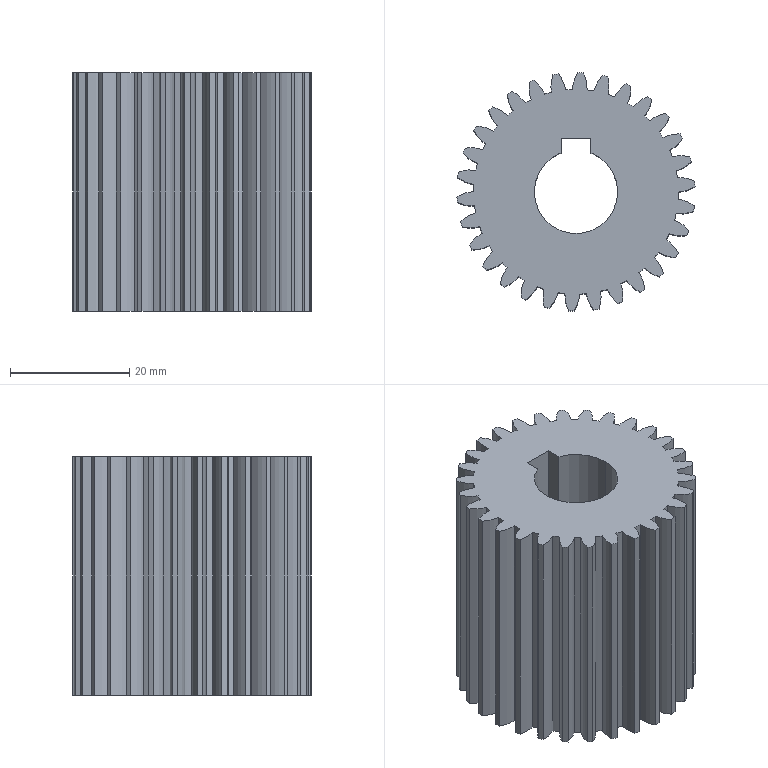Part | STEP file | External spur gear M1.25Z30 | 1 solid | 128 faces | box 39.961 x 39.996 x 40 mm | volume 37023 mm3 | cylinder 63 | spline 60 | plane 5 | commonest cylinder face diameters 34.375 x30 40 x30 14 x3